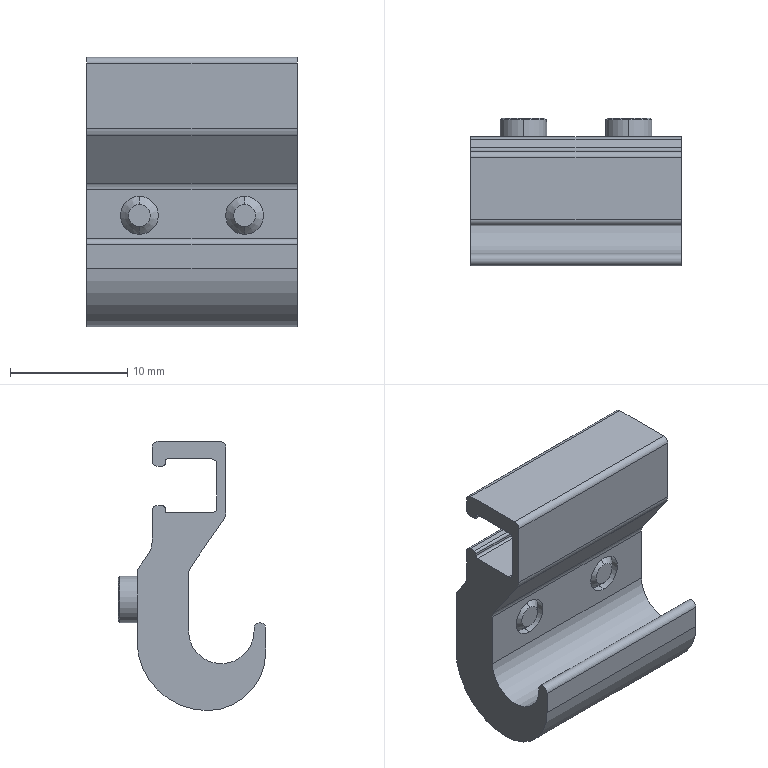Part | SolidWorks | features BaseBody 1 | 1 solid | 71 faces | box 18 x 12.6 x 23 mm | volume 2035 mm3 | plane 37 | cylinder 26 | cone 8 | commonest cylinder face diameters 4 x5 0.4 x4 0.8 x4 3.242 x4 1 x3 2 x3